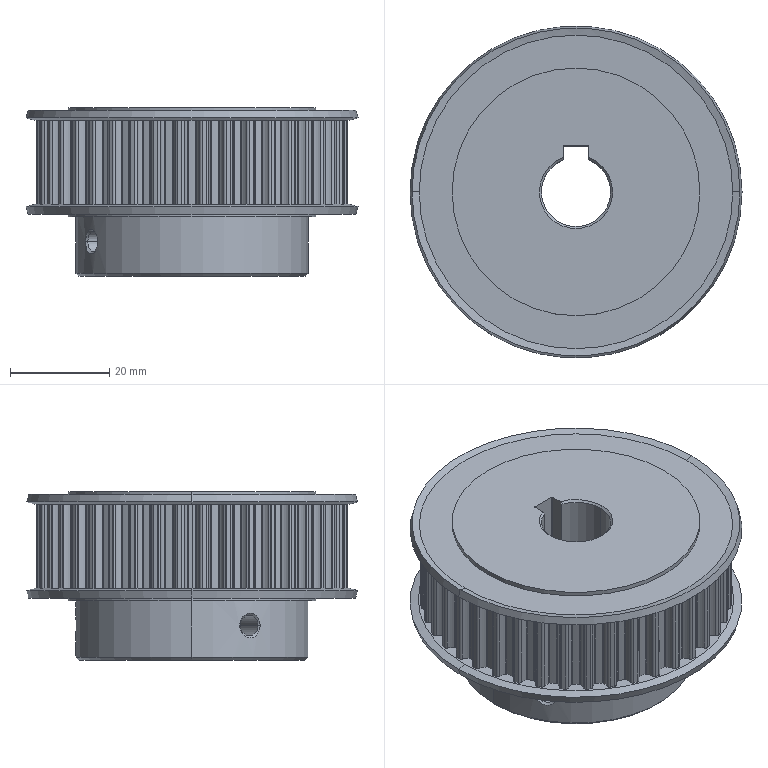Part | STEP file | 001-010-EBJ22-S5M150-40-B-N-d14 | 1 solid | 406 faces | box 67 x 67 x 34 mm | volume 78726 mm3 | cylinder 372 | cone 24 | plane 10 | commonest cylinder face diameters 1.1 x98 0.5 x92 6.55 x86 59.16 x41 62.7 x40 4.134 x4